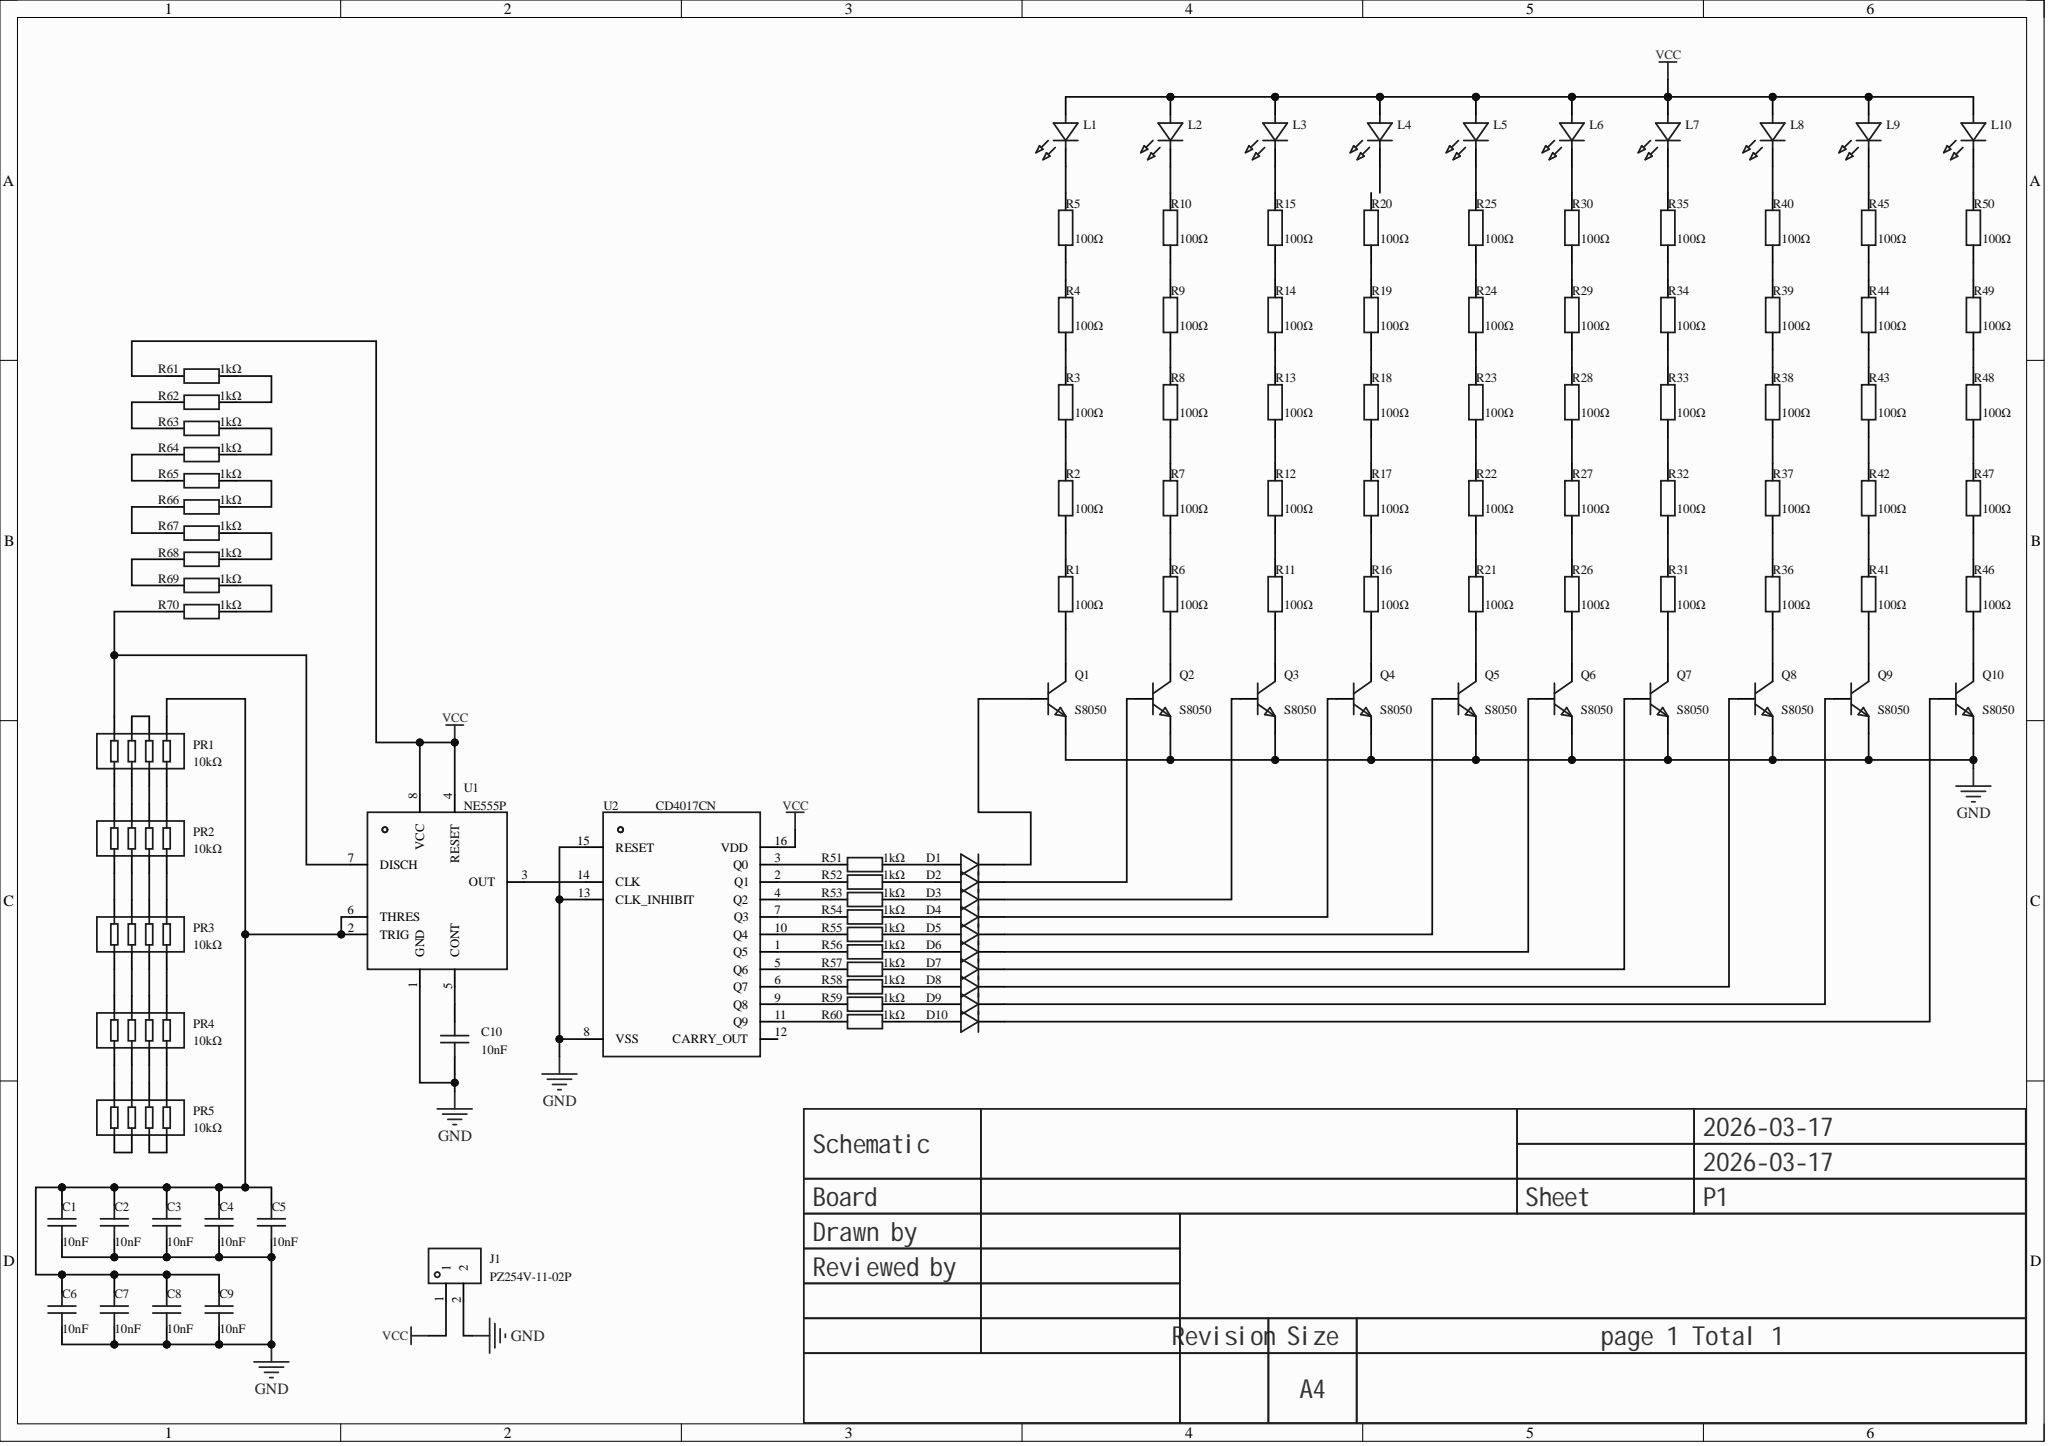Circuit board | Altium Designer | 118 parts | 123 nets
Bill of materials:
Comment,Description,Designator,Footprint,LibRef,Quantity
"10nF","Capacitance: 10nF; tolerance: ±20%; rated voltage: 1kV; temperature coefficient: Y5V;","C1, C2, C3, C4, C5, C6, C7, C8, C9, C10","CAP-TH_L8.0-W2.8-P5.08-D0.6","CC3A103MC1IEF48C30MF","10"
"1N4148TR","Diode configuration: -; forward voltage (Vf): 1V@10mA; DC reverse voltage (Vr): 100V; rectified current: 200mA; reverse recovery time (Trr): 4ns;","D1, D2, D3, D4, D5, D6, D7, D8, D9, D10","DO-35_BD2.0-L4.2-P8.20-D0.5-RD","1N4148TR_C84410","10"
"PZ254V-11-02P","Pin structure: 1x2P; pitch: 2.54mm; row spacing: -; round/square pin: square pin; mounting: through-hole; rows: single row; total pins: 2P; rated current: 3A; rated voltage: 250V; mating pin length: 6mm; housing height: 2.5mm; tail pin length: 3mm; contact material: brass; contact plating: -; operating temperature: -40℃~+105℃; color: black;","J1","HDR-TH_2P-P2.54-V-M","PZ254V-11-02P","1"
"XL-502SURD","Lamp holder type: 5mm round lamp holder; luminous color: red; forward voltage (Vf): 2.4V; power: 70mW; forward current: 20mA; wavelength: 615nm~625nm; diode configuration: -; lens color: red lens; color temperature: -; luminous intensity: 300mcd; viewing angle: 35°; tape and reel: -; operating temperature: -25℃~+85℃;","L1, L2, L3, L4, L5, L6, L7, L8, L9, L10","LED-TH_BD5.9-P2.54-RD_RED","XL-502SURD","10"
"10kΩ","Number of resistors: 4; resistance: 10kΩ; tolerance: ±2%; power per element: 300mW; temperature coefficient: ±100ppm/?;","PR1, PR2, PR3, PR4, PR5","RES-ARRAY-TH_8P-L20.3-W2.5-P2.54","4608X-102-103LF","5"
"S8050","Transistor type: NPN; collector current (Ic): 500mA; collector-emitter breakdown voltage (Vceo): 25V; power dissipation (Pd): 625mW; DC current gain (hFE): 160@50mA,1V;","Q1, Q2, Q3, Q4, Q5, Q6, Q7, Q8, Q9, Q10","TO-92-3_L4.5-W3.5-P1.27-L","S8050_C2931492","10"
"100Ω","Resistor type: metal film resistor; resistance: 100Ω; tolerance: ±1%; power: 250mW; temperature coefficient: ±50ppm/?;","R1, R2, R3, R4, R5, R6, R7, R8, R9, R10, R11, R12, R13, R14, R15, R16, R17, R18, R19, R20, R21, R22, R23, R24, R25, R26, R27, R28, R29, R30, R31, R32, R33, R34, R35, R36, R37, R38, R39, R40, R41, R42, R43, R44, R45, R46, R47, R48, R49, R50","RES-TH_BD2.2-L6.5-P10.50-D0.6","MFR0W4F1000A50","50"
"1kΩ","Resistor type: metal film resistor; resistance: 1kΩ; tolerance: ±1%; power: 250mW; temperature coefficient: ±50ppm/?;","R51, R52, R53, R54, R55, R56, R57, R58, R59, R60, R61, R62, R63, R64, R65, R66, R67, R68, R69, R70","RES-TH_BD2.5-L6.5-P10.50-D0.6","MFR0W4F1001A50","20"
"NE555P","These devices are precision timing circuits that generate accurate time delays or oscillation. In delay or monostable mode, the timing interval is set by a single external resistor and capacitor network. In astable mode, frequency and duty cycle are controlled separately by two external resistors and one external capacitor.","U1","DIP-8_L9.8-W6.6-P2.54-LS7.6-BL","NE555P","1"
"CD4017CN","CD4017BE upgraded replacement, sample recommended; 5-stage Johnson decade counter","U2","PDIP-16_L19.3-W6.4-P2.54-LS7.94-BL","CD4017CN","1"
Netlist (Protel format):
[
C1
CAP-TH_L8.0-W2.8-P5.08-D0.6
10nF



]
[
C2
CAP-TH_L8.0-W2.8-P5.08-D0.6
10nF



]
[
C3
CAP-TH_L8.0-W2.8-P5.08-D0.6
10nF



]
[
C4
CAP-TH_L8.0-W2.8-P5.08-D0.6
10nF



]
[
C5
CAP-TH_L8.0-W2.8-P5.08-D0.6
10nF



]
[
C6
CAP-TH_L8.0-W2.8-P5.08-D0.6
10nF



]
[
C7
CAP-TH_L8.0-W2.8-P5.08-D0.6
10nF



]
[
C8
CAP-TH_L8.0-W2.8-P5.08-D0.6
10nF



]
[
C9
CAP-TH_L8.0-W2.8-P5.08-D0.6
10nF



]
[
C10
CAP-TH_L8.0-W2.8-P5.08-D0.6
10nF



]
[
D1
DO-35_BD2.0-L4.2-P8.20-D0.5-RD
1N4148TR



]
[
D2
DO-35_BD2.0-L4.2-P8.20-D0.5-RD
1N4148TR



]
[
D3
DO-35_BD2.0-L4.2-P8.20-D0.5-RD
1N4148TR



]
[
D4
DO-35_BD2.0-L4.2-P8.20-D0.5-RD
1N4148TR



]
[
D5
DO-35_BD2.0-L4.2-P8.20-D0.5-RD
1N4148TR



]
[
D6
DO-35_BD2.0-L4.2-P8.20-D0.5-RD
1N4148TR



]
[
D7
DO-35_BD2.0-L4.2-P8.20-D0.5-RD
1N4148TR



]
[
D8
DO-35_BD2.0-L4.2-P8.20-D0.5-RD
1N4148TR



]
[
D9
DO-35_BD2.0-L4.2-P8.20-D0.5-RD
1N4148TR



]
[
D10
DO-35_BD2.0-L4.2-P8.20-D0.5-RD
1N4148TR



]
[
J1
HDR-TH_2P-P2.54-V-M
PZ254V-11-02P



]
[
L1
LED-TH_BD5.9-P2.54-RD_RED
XL-502SURD



]
[
L2
LED-TH_BD5.9-P2.54-RD_RED
XL-502SURD



]
[
L3
LED-TH_BD5.9-P2.54-RD_RED
XL-502SURD



]
[
L4
LED-TH_BD5.9-P2.54-RD_RED
XL-502SURD



]
[
L5
LED-TH_BD5.9-P2.54-RD_RED
XL-502SURD



]
[
L6
LED-TH_BD5.9-P2.54-RD_RED
XL-502SURD



]
[
L7
LED-TH_BD5.9-P2.54-RD_RED
XL-502SURD



]
[
L8
LED-TH_BD5.9-P2.54-RD_RED
XL-502SURD



]
[
L9
LED-TH_BD5.9-P2.54-RD_RED
XL-502SURD



]
[
L10
LED-TH_BD5.9-P2.54-RD_RED
XL-502SURD



]
[
PR1
RES-ARRAY-TH_8P-L20.3-W2.5-P2.54
10kΩ



]
[
PR2
RES-ARRAY-TH_8P-L20.3-W2.5-P2.54
10kΩ



]
[
PR3
RES-ARRAY-TH_8P-L20.3-W2.5-P2.54
10kΩ



]
[
PR4
RES-ARRAY-TH_8P-L20.3-W2.5-P2.54
10kΩ



]
[
PR5
RES-ARRAY-TH_8P-L20.3-W2.5-P2.54
10kΩ



]
[
Q1
TO-92-3_L4.5-W3.5-P1.27-L
S8050



]
[
Q2
TO-92-3_L4.5-W3.5-P1.27-L
S8050



]
[
Q3
TO-92-3_L4.5-W3.5-P1.27-L
S8050



]
[
Q4
TO-92-3_L4.5-W3.5-P1.27-L
S8050



]
[
Q5
TO-92-3_L4.5-W3.5-P1.27-L
S8050



]
[
Q6
TO-92-3_L4.5-W3.5-P1.27-L
S8050



]
[
Q7
TO-92-3_L4.5-W3.5-P1.27-L
S8050



]
[
Q8
TO-92-3_L4.5-W3.5-P1.27-L
S8050



]
[
Q9
TO-92-3_L4.5-W3.5-P1.27-L
S8050



]
[
Q10
TO-92-3_L4.5-W3.5-P1.27-L
S8050



]
[
R1
RES-TH_BD2.2-L6.5-P10.50-D0.6
100Ω



]
[
R2
RES-TH_BD2.2-L6.5-P10.50-D0.6
100Ω



]
[
R3
RES-TH_BD2.2-L6.5-P10.50-D0.6
100Ω



]
[
R4
RES-TH_BD2.2-L6.5-P10.50-D0.6
100Ω



]
[
R5
RES-TH_BD2.2-L6.5-P10.50-D0.6
100Ω



]
[
R6
RES-TH_BD2.2-L6.5-P10.50-D0.6
100Ω



]
[
R7
RES-TH_BD2.2-L6.5-P10.50-D0.6
100Ω



]
[
R8
RES-TH_BD2.2-L6.5-P10.50-D0.6
100Ω



]
[
R9
RES-TH_BD2.2-L6.5-P10.50-D0.6
100Ω



]
[
R10
RES-TH_BD2.2-L6.5-P10.50-D0.6
100Ω



]
[
R11
RES-TH_BD2.2-L6.5-P10.50-D0.6
100Ω



]
[
R12
RES-TH_BD2.2-L6.5-P10.50-D0.6
100Ω



]
[
R13
RES-TH_BD2.2-L6.5-P10.50-D0.6
100Ω



]
[
R14
RES-TH_BD2.2-L6.5-P10.50-D0.6
100Ω



]
[
R15
RES-TH_BD2.2-L6.5-P10.50-D0.6
100Ω



]
[
R16
RES-TH_BD2.2-L6.5-P10.50-D0.6
100Ω



]
[
R17
RES-TH_BD2.2-L6.5-P10.50-D0.6
100Ω



]
[
R18
RES-TH_BD2.2-L6.5-P10.50-D0.6
100Ω



]
[
R19
RES-TH_BD2.2-L6.5-P10.50-D0.6
100Ω



]
[
R20
RES-TH_BD2.2-L6.5-P10.50-D0.6
100Ω



]
[
R21
RES-TH_BD2.2-L6.5-P10.50-D0.6
100Ω



]
[
R22
RES-TH_BD2.2-L6.5-P10.50-D0.6
100Ω



]
[
R23
RES-TH_BD2.2-L6.5-P10.50-D0.6
100Ω



]
[
R24
RES-TH_BD2.2-L6.5-P10.50-D0.6
100Ω



]
[
R25
RES-TH_BD2.2-L6.5-P10.50-D0.6
100Ω



]
[
R26
RES-TH_BD2.2-L6.5-P10.50-D0.6
100Ω



]
[
R27
RES-TH_BD2.2-L6.5-P10.50-D0.6
100Ω



]
[
R28
RES-TH_BD2.2-L6.5-P10.50-D0.6
100Ω



]
[
R29
RES-TH_BD2.2-L6.5-P10.50-D0.6
100Ω



]
[
R30
RES-TH_BD2.2-L6.5-P10.50-D0.6
100Ω



]
[
R31
RES-TH_BD2.2-L6.5-P10.50-D0.6
100Ω



]
[
R32
RES-TH_BD2.2-L6.5-P10.50-D0.6
100Ω



]
[
R33
RES-TH_BD2.2-L6.5-P10.50-D0.6
100Ω



]
[
R34
RES-TH_BD2.2-L6.5-P10.50-D0.6
100Ω



]
[
R35
RES-TH_BD2.2-L6.5-P10.50-D0.6
100Ω



]
[
R36
RES-TH_BD2.2-L6.5-P10.50-D0.6
100Ω



]
[
R37
RES-TH_BD2.2-L6.5-P10.50-D0.6
100Ω



]
[
R38
RES-TH_BD2.2-L6.5-P10.50-D0.6
100Ω



]
[
R39
RES-TH_BD2.2-L6.5-P10.50-D0.6
100Ω



]
[
R40
RES-TH_BD2.2-L6.5-P10.50-D0.6
100Ω



]
[
R41
RES-TH_BD2.2-L6.5-P10.50-D0.6
100Ω



]
[
R42
RES-TH_BD2.2-L6.5-P10.50-D0.6
100Ω



]
[
R43
RES-TH_BD2.2-L6.5-P10.50-D0.6
100Ω



]
[
R44
RES-TH_BD2.2-L6.5-P10.50-D0.6
100Ω



]
[
R45
RES-TH_BD2.2-L6.5-P10.50-D0.6
100Ω



]
[
R46
RES-TH_BD2.2-L6.5-P10.50-D0.6
100Ω



]
[
R47
RES-TH_BD2.2-L6.5-P10.50-D0.6
100Ω



]
[
R48
RES-TH_BD2.2-L6.5-P10.50-D0.6
100Ω



]
[
R49
RES-TH_BD2.2-L6.5-P10.50-D0.6
100Ω



]
[
R50
RES-TH_BD2.2-L6.5-P10.50-D0.6
100Ω



]
[
R51
RES-TH_BD2.5-L6.5-P10.50-D0.6
1kΩ



]
[
R52
RES-TH_BD2.5-L6.5-P10.50-D0.6
1kΩ



]
[
R53
RES-TH_BD2.5-L6.5-P10.50-D0.6
1kΩ



]
[
R54
RES-TH_BD2.5-L6.5-P10.50-D0.6
1kΩ



]
[
R55
RES-TH_BD2.5-L6.5-P10.50-D0.6
1kΩ



]
[
R56
RES-TH_BD2.5-L6.5-P10.50-D0.6
1kΩ



]
[
R57
RES-TH_BD2.5-L6.5-P10.50-D0.6
1kΩ



]
[
R58
RES-TH_BD2.5-L6.5-P10.50-D0.6
1kΩ



]
[
R59
RES-TH_BD2.5-L6.5-P10.50-D0.6
1kΩ



]
[
R60
RES-TH_BD2.5-L6.5-P10.50-D0.6
1kΩ



]
[
R61
RES-TH_BD2.5-L6.5-P10.50-D0.6
1kΩ



]
[
R62
RES-TH_BD2.5-L6.5-P10.50-D0.6
1kΩ



]
[
R63
RES-TH_BD2.5-L6.5-P10.50-D0.6
1kΩ



]
[
R64
RES-TH_BD2.5-L6.5-P10.50-D0.6
1kΩ



]
[
R65
RES-TH_BD2.5-L6.5-P10.50-D0.6
1kΩ



]
[
R66
RES-TH_BD2.5-L6.5-P10.50-D0.6
1kΩ



]
[
R67
RES-TH_BD2.5-L6.5-P10.50-D0.6
1kΩ



]
[
R68
RES-TH_BD2.5-L6.5-P10.50-D0.6
1kΩ



]
[
R69
RES-TH_BD2.5-L6.5-P10.50-D0.6
1kΩ



]
[
R70
RES-TH_BD2.5-L6.5-P10.50-D0.6
1kΩ



]
[
U1
DIP-8_L9.8-W6.6-P2.54-LS7.6-BL
NE555P



]
[
U2
PDIP-16_L19.3-W6.4-P2.54-LS7.94-BL
CD4017CN



]
(
VCC
J1-1
L1-2
L2-2
L3-2
L4-2
L5-2
L6-2
L7-2
L8-2
L9-2
L10-2
R61-1
U1-4
U1-8
U2-16
)
(
NetU1_3
U1-3
U2-14
)
(
NetR69_2
R69-2
R70-2
)
(
NetR68_1
R68-1
R69-1
)
(
NetR67_2
R67-2
R68-2
)
(
NetR66_1
R66-1
R67-1
)
(
NetR65_2
R65-2
R66-2
)
(
NetR64_1
R64-1
R65-1
)
(
NetR63_2
R63-2
R64-2
)
(
NetR62_1
R62-1
R63-1
)
(
NetR61_2
R61-2
R62-2
)
(
NetR60_1
R60-1
U2-11
)
(
NetR59_1
R59-1
U2-9
)
(
NetR58_1
R58-1
U2-6
)
(
NetR57_1
R57-1
U2-5
)
(
NetR56_1
R56-1
U2-1
)
(
NetR55_1
R55-1
U2-10
)
(
NetR54_1
R54-1
U2-7
)
(
NetR53_1
R53-1
U2-4
)
(
NetR52_1
R52-1
U2-2
)
(
NetR51_1
R51-1
U2-3
)
(
NetR49_2
R49-2
R50-1
)
(
NetR48_2
R48-2
R49-1
)
(
NetR47_2
R47-2
R48-1
)
(
NetR46_2
R46-2
R47-1
)
(
NetR44_2
R44-2
R45-1
)
(
NetR43_2
R43-2
R44-1
)
(
NetR42_2
R42-2
R43-1
)
(
NetR41_2
R41-2
R42-1
)
(
NetR39_2
R39-2
R40-1
)
(
NetR38_2
R38-2
R39-1
)
(
NetR37_2
R37-2
R38-1
)
(
NetR36_2
R36-2
R37-1
)
(
NetR34_2
R34-2
R35-1
)
(
NetR33_2
R33-2
R34-1
)
(
NetR32_2
R32-2
R33-1
)
(
NetR31_2
R31-2
R32-1
)
(
NetR29_2
R29-2
R30-1
)
(
NetR28_2
R28-2
R29-1
)
(
NetR27_2
R27-2
R28-1
)
(
NetR26_2
R26-2
R27-1
)
(
NetR24_2
R24-2
R25-1
)
(
NetR23_2
R23-2
R24-1
)
(
NetR22_2
R22-2
R23-1
)
(
NetR21_2
R21-2
R22-1
)
(
NetR19_2
R19-2
R20-1
)
(
NetR18_2
R18-2
R19-1
)
(
NetR17_2
R17-2
R18-1
)
(
NetR16_2
R16-2
R17-1
)
(
NetR14_2
R14-2
R15-1
)
(
NetR13_2
R13-2
R14-1
)
(
NetR12_2
R12-2
R13-1
)
(
NetR11_2
R11-2
R12-1
)
(
NetR9_2
R9-2
R10-1
)
(
NetR8_2
R8-2
R9-1
)
(
NetR7_2
R7-2
R8-1
)
(
NetR6_2
R6-2
R7-1
)
(
NetR4_2
R4-2
R5-1
)
(
NetR3_2
R3-2
R4-1
)
(
NetR2_2
R2-2
R3-1
)
(
NetR1_2
R1-2
R2-1
)
(
NetQ10_3
Q10-3
R46-1
)
(
NetQ9_3
Q9-3
R41-1
)
(
NetQ8_3
Q8-3
R36-1
)
(
NetQ7_3
Q7-3
R31-1
)
(
NetQ6_3
Q6-3
R26-1
)
(
NetQ5_3
Q5-3
R21-1
)
(
NetQ4_3
Q4-3
R16-1
)
(
NetQ3_3
Q3-3
R11-1
)
(
NetQ2_3
Q2-3
R6-1
)
(
NetQ1_3
Q1-3
R1-1
)
(
NetPR5_3
PR5-3
PR5-4
)
(
NetPR5_1
PR5-1
PR5-2
)
(
NetPR4_4
PR4-4
PR5-5
)
(
NetPR4_3
PR4-3
PR5-6
)
(
NetPR4_2
PR4-2
PR5-7
)
(
NetPR4_1
PR4-1
PR5-8
)
(
NetPR3_4
PR3-4
PR4-5
)
(
NetPR3_3
PR3-3
PR4-6
)
(
NetPR3_2
PR3-2
PR4-7
)
(
NetPR3_1
PR3-1
PR4-8
)
(
NetPR2_4
PR2-4
PR3-5
)
(
NetPR2_3
PR2-3
PR3-6
)
(
NetPR2_2
PR2-2
PR3-7
)
(
NetPR2_1
PR2-1
PR3-8
)
(
NetPR1_8
PR1-8
R70-1
U1-7
)
(
NetPR1_6
PR1-6
PR1-7
)
(
NetPR1_4
PR1-4
PR2-5
)
(
NetPR1_3
PR1-3
PR2-6
)
(
NetPR1_2
PR1-2
PR2-7
)
(
NetPR1_1
PR1-1
PR2-8
)
(
NetL10_1
L10-1
R50-2
)
(
NetL9_1
L9-1
R45-2
)
(
NetL8_1
L8-1
R40-2
)
(
NetL7_1
L7-1
R35-2
)
(
NetL6_1
L6-1
R30-2
)
(
NetL5_1
L5-1
R25-2
)
(
NetL3_1
L3-1
R15-2
)
(
NetL2_1
L2-1
R10-2
)
(
NetL1_1
L1-1
R5-2
)
(
NetD10_2
D10-2
R60-2
)
(
NetD10_1
D10-1
Q10-2
)
(
NetD9_2
D9-2
R59-2
)
(
NetD9_1
D9-1
Q9-2
)
(
NetD8_2
D8-2
R58-2
)
(
NetD8_1
D8-1
Q8-2
)
(
NetD7_2
D7-2
R57-2
)
(
NetD7_1
D7-1
Q7-2
)
(
NetD6_2
D6-2
R56-2
)
(
NetD6_1
D6-1
Q6-2
)
(
NetD5_2
D5-2
R55-2
)
(
NetD5_1
D5-1
Q5-2
)
(
NetD4_2
D4-2
R54-2
)
(
NetD4_1
D4-1
Q4-2
)
(
NetD3_2
D3-2
R53-2
)
(
NetD3_1
D3-1
Q3-2
)
(
NetD2_2
D2-2
R52-2
)
(
NetD2_1
D2-1
Q2-2
)
(
NetD1_2
D1-2
R51-2
)
(
NetD1_1
D1-1
Q1-2
)
(
NetC10_2
C10-2
U1-5
)
(
NetC1_2
C1-2
C2-2
C3-2
C4-2
C5-2
C6-2
C7-2
C8-2
C9-2
PR1-5
U1-2
U1-6
)
(
GND
C1-1
C2-1
C3-1
C4-1
C5-1
C6-1
C7-1
C8-1
C9-1
C10-1
J1-2
Q1-1
Q2-1
Q3-1
Q4-1
Q5-1
Q6-1
Q7-1
Q8-1
Q9-1
Q10-1
U1-1
U2-8
U2-13
U2-15
)